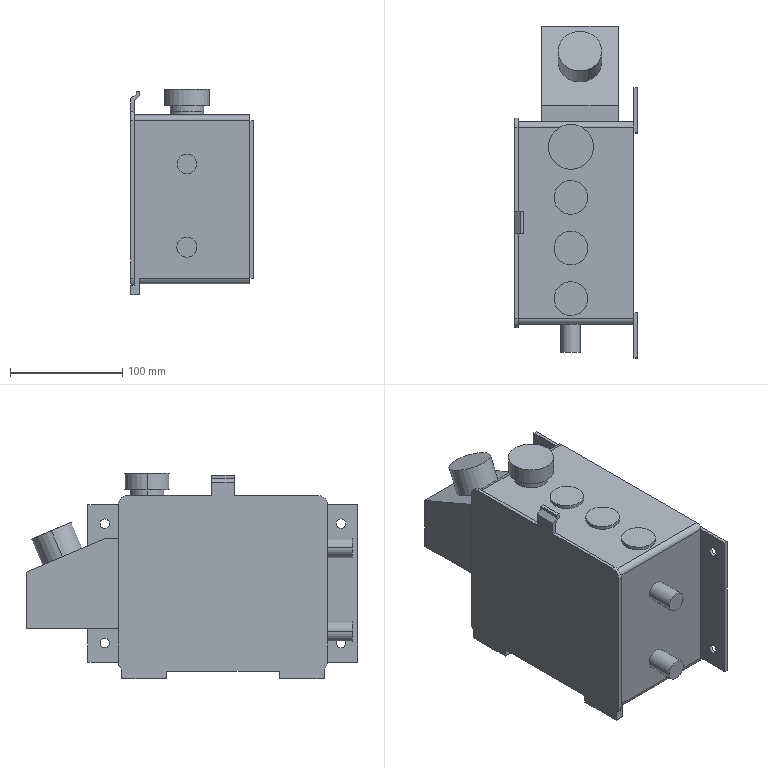Part | NX | features .1 2 | 1 solid | 84 faces | box 109 x 295 x 183 mm | volume 3368077 mm3 | plane 52 | cylinder 28 | spline 4 | commonest cylinder face diameters 8.5 x8 30 x8 10 x4 17.341 x2 17.971 x2 38.5 x2